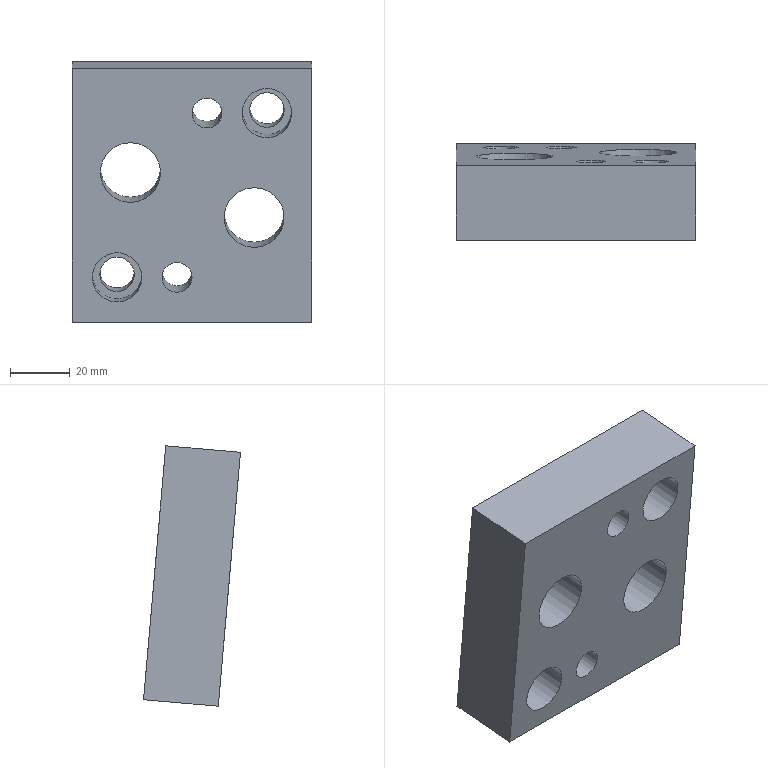Part | NX | features solid 2 | 1 solid | 20 faces | box 80 x 32.313 x 86.855 mm | volume 140365 mm3 | plane 10 | cylinder 10 | commonest cylinder face diameters 10 x2 11.5 x2 16.5 x2 20 x2 26 x2
STEP:
#1=CARTESIAN_POINT('',(208.,113.182,11.018));
#2=VERTEX_POINT('',#1);
#3=CARTESIAN_POINT('',(128.,113.182,11.018));
#4=VERTEX_POINT('',#3);
#5=CARTESIAN_POINT('',(208.,113.182,11.018));
#6=DIRECTION('',(-1.,0.,0.));
#7=VECTOR('',#6,1000.);
#8=LINE('',#5,#7);
#9=EDGE_CURVE('',#2,#4,#8,.T.);
#10=ORIENTED_EDGE('',*,*,#9,.F.);
#11=CARTESIAN_POINT('',(208.,138.087,13.197));
#12=VERTEX_POINT('',#11);
#13=CARTESIAN_POINT('',(208.,143.068,13.633));
#14=DIRECTION('',(0.,0.9962,0.08716));
#15=VECTOR('',#14,1000.);
#16=LINE('',#13,#15);
#17=EDGE_CURVE('',#12,#2,#16,.F.);
#18=ORIENTED_EDGE('',*,*,#17,.F.);
#19=CARTESIAN_POINT('',(128.,138.087,13.197));
#20=VERTEX_POINT('',#19);
#21=CARTESIAN_POINT('',(208.,138.087,13.197));
#22=DIRECTION('',(-1.,0.,0.));
#23=VECTOR('',#22,1000.);
#24=LINE('',#21,#23);
#25=EDGE_CURVE('',#12,#20,#24,.T.);
#26=ORIENTED_EDGE('',*,*,#25,.T.);
#27=CARTESIAN_POINT('',(128.,138.087,13.197));
#28=DIRECTION('',(0.,0.9962,0.08716));
#29=VECTOR('',#28,1000.);
#30=LINE('',#27,#29);
#31=EDGE_CURVE('',#20,#4,#30,.F.);
#32=ORIENTED_EDGE('',*,*,#31,.T.);
#33=EDGE_LOOP('',(#10,#18,#26,#32));
#34=FACE_BOUND('',#33,.T.);
#35=CARTESIAN_POINT('',(208.,143.068,13.633));
#36=DIRECTION('',(0.,0.08716,-0.9962));
#37=DIRECTION('',(0.,0.9962,0.08716));
#38=AXIS2_PLACEMENT_3D('',#35,#36,#37);
#39=PLANE('',#38);
#40=ADVANCED_FACE('',(#34),#39,.F.);
#41=CARTESIAN_POINT('',(128.,120.59,-73.658));
#42=VERTEX_POINT('',#41);
#43=CARTESIAN_POINT('',(128.,113.063,12.385));
#44=DIRECTION('',(0.,0.08716,-0.9962));
#45=VECTOR('',#44,1000.);
#46=LINE('',#43,#45);
#47=EDGE_CURVE('',#42,#4,#46,.F.);
#48=ORIENTED_EDGE('',*,*,#47,.T.);
#49=ORIENTED_EDGE('',*,*,#31,.F.);
#50=CARTESIAN_POINT('',(128.,145.495,-71.479));
#51=VERTEX_POINT('',#50);
#52=CARTESIAN_POINT('',(128.,137.967,14.563));
#53=DIRECTION('',(0.,0.08716,-0.9962));
#54=VECTOR('',#53,1000.);
#55=LINE('',#52,#54);
#56=EDGE_CURVE('',#51,#20,#55,.F.);
#57=ORIENTED_EDGE('',*,*,#56,.F.);
#58=CARTESIAN_POINT('',(128.,145.495,-71.479));
#59=DIRECTION('',(0.,0.9962,0.08716));
#60=VECTOR('',#59,1000.);
#61=LINE('',#58,#60);
#62=EDGE_CURVE('',#51,#42,#61,.F.);
#63=ORIENTED_EDGE('',*,*,#62,.T.);
#64=EDGE_LOOP('',(#48,#49,#57,#63));
#65=FACE_BOUND('',#64,.T.);
#66=CARTESIAN_POINT('',(128.,137.967,14.563));
#67=DIRECTION('',(1.,0.,0.));
#68=DIRECTION('',(0.,0.,-1.));
#69=AXIS2_PLACEMENT_3D('',#66,#67,#68);
#70=PLANE('',#69);
#71=ADVANCED_FACE('',(#65),#70,.F.);
#72=CARTESIAN_POINT('',(208.,120.59,-73.658));
#73=VERTEX_POINT('',#72);
#74=CARTESIAN_POINT('',(171.,120.59,-73.658));
#75=DIRECTION('',(1.,0.,0.));
#76=VECTOR('',#75,1000.);
#77=LINE('',#74,#76);
#78=EDGE_CURVE('',#42,#73,#77,.T.);
#79=ORIENTED_EDGE('',*,*,#78,.F.);
#80=ORIENTED_EDGE('',*,*,#62,.F.);
#81=CARTESIAN_POINT('',(208.,145.495,-71.479));
#82=VERTEX_POINT('',#81);
#83=CARTESIAN_POINT('',(171.,145.495,-71.479));
#84=DIRECTION('',(1.,0.,0.));
#85=VECTOR('',#84,1000.);
#86=LINE('',#83,#85);
#87=EDGE_CURVE('',#51,#82,#86,.T.);
#88=ORIENTED_EDGE('',*,*,#87,.T.);
#89=CARTESIAN_POINT('',(208.,279.982,-59.713));
#90=DIRECTION('',(0.,0.9962,0.08716));
#91=VECTOR('',#90,1000.);
#92=LINE('',#89,#91);
#93=EDGE_CURVE('',#82,#73,#92,.F.);
#94=ORIENTED_EDGE('',*,*,#93,.T.);
#95=EDGE_LOOP('',(#79,#80,#88,#94));
#96=FACE_BOUND('',#95,.T.);
#97=CARTESIAN_POINT('',(171.,279.982,-59.713));
#98=DIRECTION('',(0.,0.08716,-0.9962));
#99=DIRECTION('',(-1.,0.,0.));
#100=AXIS2_PLACEMENT_3D('',#97,#98,#99);
#101=PLANE('',#100);
#102=ADVANCED_FACE('',(#96),#101,.T.);
#103=CARTESIAN_POINT('',(208.,113.063,12.385));
#104=DIRECTION('',(0.,-0.08716,0.9962));
#105=VECTOR('',#104,1000.);
#106=LINE('',#103,#105);
#107=EDGE_CURVE('',#2,#73,#106,.F.);
#108=ORIENTED_EDGE('',*,*,#107,.T.);
#109=ORIENTED_EDGE('',*,*,#93,.F.);
#110=CARTESIAN_POINT('',(208.,142.543,-37.735));
#111=DIRECTION('',(0.,0.08716,-0.9962));
#112=VECTOR('',#111,1000.);
#113=LINE('',#110,#112);
#114=EDGE_CURVE('',#12,#82,#113,.T.);
#115=ORIENTED_EDGE('',*,*,#114,.F.);
#116=ORIENTED_EDGE('',*,*,#17,.T.);
#117=EDGE_LOOP('',(#108,#109,#115,#116));
#118=FACE_BOUND('',#117,.T.);
#119=CARTESIAN_POINT('',(208.,142.543,-37.735));
#120=DIRECTION('',(-1.,0.,0.));
#121=DIRECTION('',(0.,0.,1.));
#122=AXIS2_PLACEMENT_3D('',#119,#120,#121);
#123=PLANE('',#122);
#124=ADVANCED_FACE('',(#118),#123,.F.);
#125=CARTESIAN_POINT('',(193.,138.893,3.982));
#126=VERTEX_POINT('',#125);
#127=CARTESIAN_POINT('',(193.,139.394,-1.746));
#128=DIRECTION('',(0.,0.9962,0.08716));
#129=DIRECTION('',(0.,-0.08716,0.9962));
#130=AXIS2_PLACEMENT_3D('',#127,#128,#129);
#131=CIRCLE('',#130,5.75);
#132=EDGE_CURVE('',#126,#126,#131,.F.);
#133=ORIENTED_EDGE('',*,*,#132,.T.);
#134=EDGE_LOOP('',(#133));
#135=FACE_BOUND('',#134,.T.);
#136=CARTESIAN_POINT('',(173.,138.959,3.235));
#137=VERTEX_POINT('',#136);
#138=CARTESIAN_POINT('',(173.,139.394,-1.746));
#139=DIRECTION('',(0.,0.9962,0.08716));
#140=DIRECTION('',(0.,-0.08716,0.9962));
#141=AXIS2_PLACEMENT_3D('',#138,#139,#140);
#142=CIRCLE('',#141,5.);
#143=EDGE_CURVE('',#137,#137,#142,.F.);
#144=ORIENTED_EDGE('',*,*,#143,.T.);
#145=EDGE_LOOP('',(#144));
#146=FACE_BOUND('',#145,.T.);
#147=CARTESIAN_POINT('',(163.,143.752,-51.556));
#148=VERTEX_POINT('',#147);
#149=CARTESIAN_POINT('',(163.,144.188,-56.537));
#150=DIRECTION('',(0.,0.9962,0.08716));
#151=DIRECTION('',(0.,-0.08716,0.9962));
#152=AXIS2_PLACEMENT_3D('',#149,#150,#151);
#153=CIRCLE('',#152,5.);
#154=EDGE_CURVE('',#148,#148,#153,.F.);
#155=ORIENTED_EDGE('',*,*,#154,.T.);
#156=EDGE_LOOP('',(#155));
#157=FACE_BOUND('',#156,.T.);
#158=CARTESIAN_POINT('',(143.,143.687,-50.808));
#159=VERTEX_POINT('',#158);
#160=CARTESIAN_POINT('',(143.,144.188,-56.537));
#161=DIRECTION('',(0.,0.9962,0.08716));
#162=DIRECTION('',(0.,-0.08716,0.9962));
#163=AXIS2_PLACEMENT_3D('',#160,#161,#162);
#164=CIRCLE('',#163,5.75);
#165=EDGE_CURVE('',#159,#159,#164,.F.);
#166=ORIENTED_EDGE('',*,*,#165,.T.);
#167=EDGE_LOOP('',(#166));
#168=FACE_BOUND('',#167,.T.);
#169=CARTESIAN_POINT('',(147.466,139.995,-8.608));
#170=VERTEX_POINT('',#169);
#171=CARTESIAN_POINT('',(147.466,141.128,-21.558));
#172=DIRECTION('',(0.,0.9962,0.08716));
#173=DIRECTION('',(0.,-0.08716,0.9962));
#174=AXIS2_PLACEMENT_3D('',#171,#172,#173);
#175=CIRCLE('',#174,13.);
#176=EDGE_CURVE('',#170,#170,#175,.F.);
#177=ORIENTED_EDGE('',*,*,#176,.T.);
#178=EDGE_LOOP('',(#177));
#179=FACE_BOUND('',#178,.T.);
#180=CARTESIAN_POINT('',(188.737,141.307,-23.61));
#181=VERTEX_POINT('',#180);
#182=CARTESIAN_POINT('',(188.737,142.44,-36.56));
#183=DIRECTION('',(0.,0.9962,0.08716));
#184=DIRECTION('',(0.,-0.08716,0.9962));
#185=AXIS2_PLACEMENT_3D('',#182,#183,#184);
#186=CIRCLE('',#185,13.);
#187=EDGE_CURVE('',#181,#181,#186,.F.);
#188=ORIENTED_EDGE('',*,*,#187,.T.);
#189=EDGE_LOOP('',(#188));
#190=FACE_BOUND('',#189,.T.);
#191=ORIENTED_EDGE('',*,*,#25,.F.);
#192=ORIENTED_EDGE('',*,*,#114,.T.);
#193=ORIENTED_EDGE('',*,*,#87,.F.);
#194=ORIENTED_EDGE('',*,*,#56,.T.);
#195=EDGE_LOOP('',(#191,#192,#193,#194));
#196=FACE_BOUND('',#195,.T.);
#197=CARTESIAN_POINT('',(208.,137.967,14.563));
#198=DIRECTION('',(0.,0.9962,0.08716));
#199=DIRECTION('',(-1.,0.,0.));
#200=AXIS2_PLACEMENT_3D('',#197,#198,#199);
#201=PLANE('',#200);
#202=ADVANCED_FACE('',(#135,#146,#157,#168,#179,#190,#196),#201,.T.);
#203=CARTESIAN_POINT('',(178.,114.489,-3.925));
#204=VERTEX_POINT('',#203);
#205=CARTESIAN_POINT('',(173.,114.489,-3.925));
#206=DIRECTION('',(0.,0.9962,0.08716));
#207=DIRECTION('',(1.,0.,0.));
#208=AXIS2_PLACEMENT_3D('',#205,#206,#207);
#209=CIRCLE('',#208,5.);
#210=EDGE_CURVE('',#204,#204,#209,.T.);
#211=ORIENTED_EDGE('',*,*,#210,.T.);
#212=EDGE_LOOP('',(#211));
#213=FACE_BOUND('',#212,.T.);
#214=CARTESIAN_POINT('',(168.,119.283,-58.715));
#215=VERTEX_POINT('',#214);
#216=CARTESIAN_POINT('',(163.,119.283,-58.715));
#217=DIRECTION('',(0.,0.9962,0.08716));
#218=DIRECTION('',(1.,0.,0.));
#219=AXIS2_PLACEMENT_3D('',#216,#217,#218);
#220=CIRCLE('',#219,5.);
#221=EDGE_CURVE('',#215,#215,#220,.T.);
#222=ORIENTED_EDGE('',*,*,#221,.T.);
#223=EDGE_LOOP('',(#222));
#224=FACE_BOUND('',#223,.T.);
#225=CARTESIAN_POINT('',(151.25,119.283,-58.715));
#226=VERTEX_POINT('',#225);
#227=CARTESIAN_POINT('',(143.,119.283,-58.715));
#228=DIRECTION('',(0.,0.9962,0.08716));
#229=DIRECTION('',(1.,0.,0.));
#230=AXIS2_PLACEMENT_3D('',#227,#228,#229);
#231=CIRCLE('',#230,8.25);
#232=EDGE_CURVE('',#226,#226,#231,.T.);
#233=ORIENTED_EDGE('',*,*,#232,.T.);
#234=EDGE_LOOP('',(#233));
#235=FACE_BOUND('',#234,.T.);
#236=CARTESIAN_POINT('',(201.25,114.489,-3.925));
#237=VERTEX_POINT('',#236);
#238=CARTESIAN_POINT('',(193.,114.489,-3.925));
#239=DIRECTION('',(0.,0.9962,0.08716));
#240=DIRECTION('',(1.,0.,0.));
#241=AXIS2_PLACEMENT_3D('',#238,#239,#240);
#242=CIRCLE('',#241,8.25);
#243=EDGE_CURVE('',#237,#237,#242,.T.);
#244=ORIENTED_EDGE('',*,*,#243,.T.);
#245=EDGE_LOOP('',(#244));
#246=FACE_BOUND('',#245,.T.);
#247=CARTESIAN_POINT('',(147.466,115.351,-13.775));
#248=VERTEX_POINT('',#247);
#249=CARTESIAN_POINT('',(147.466,116.223,-23.737));
#250=DIRECTION('',(0.,0.9962,0.08716));
#251=DIRECTION('',(0.,-0.08716,0.9962));
#252=AXIS2_PLACEMENT_3D('',#249,#250,#251);
#253=CIRCLE('',#252,10.);
#254=EDGE_CURVE('',#248,#248,#253,.F.);
#255=ORIENTED_EDGE('',*,*,#254,.F.);
#256=EDGE_LOOP('',(#255));
#257=FACE_BOUND('',#256,.T.);
#258=CARTESIAN_POINT('',(188.737,116.664,-28.777));
#259=VERTEX_POINT('',#258);
#260=CARTESIAN_POINT('',(188.737,117.535,-38.739));
#261=DIRECTION('',(0.,0.9962,0.08716));
#262=DIRECTION('',(0.,-0.08716,0.9962));
#263=AXIS2_PLACEMENT_3D('',#260,#261,#262);
#264=CIRCLE('',#263,10.);
#265=EDGE_CURVE('',#259,#259,#264,.F.);
#266=ORIENTED_EDGE('',*,*,#265,.F.);
#267=EDGE_LOOP('',(#266));
#268=FACE_BOUND('',#267,.T.);
#269=ORIENTED_EDGE('',*,*,#9,.T.);
#270=ORIENTED_EDGE('',*,*,#47,.F.);
#271=ORIENTED_EDGE('',*,*,#78,.T.);
#272=ORIENTED_EDGE('',*,*,#107,.F.);
#273=EDGE_LOOP('',(#269,#270,#271,#272));
#274=FACE_BOUND('',#273,.T.);
#275=CARTESIAN_POINT('',(208.,113.063,12.385));
#276=DIRECTION('',(0.,0.9962,0.08716));
#277=DIRECTION('',(-1.,0.,0.));
#278=AXIS2_PLACEMENT_3D('',#275,#276,#277);
#279=PLANE('',#278);
#280=ADVANCED_FACE('',(#213,#224,#235,#246,#257,#268,#274),#279,.F.);
#281=ORIENTED_EDGE('',*,*,#265,.T.);
#282=EDGE_LOOP('',(#281));
#283=FACE_BOUND('',#282,.T.);
#284=CARTESIAN_POINT('',(188.737,138.331,-46.958));
#285=VERTEX_POINT('',#284);
#286=CARTESIAN_POINT('',(188.737,137.459,-36.996));
#287=DIRECTION('',(0.,-0.9962,-0.08716));
#288=DIRECTION('',(0.,0.08716,-0.9962));
#289=AXIS2_PLACEMENT_3D('',#286,#287,#288);
#290=CIRCLE('',#289,10.);
#291=EDGE_CURVE('',#285,#285,#290,.F.);
#292=ORIENTED_EDGE('',*,*,#291,.T.);
#293=EDGE_LOOP('',(#292));
#294=FACE_BOUND('',#293,.T.);
#295=CARTESIAN_POINT('',(188.737,75.948,-42.378));
#296=DIRECTION('',(0.,0.9962,0.08716));
#297=DIRECTION('',(0.,-0.08716,0.9962));
#298=AXIS2_PLACEMENT_3D('',#295,#296,#297);
#299=CYLINDRICAL_SURFACE('',#298,10.);
#300=ADVANCED_FACE('',(#283,#294),#299,.F.);
#301=ORIENTED_EDGE('',*,*,#291,.F.);
#302=EDGE_LOOP('',(#301));
#303=FACE_BOUND('',#302,.T.);
#304=CARTESIAN_POINT('',(175.737,137.459,-36.996));
#305=VERTEX_POINT('',#304);
#306=CARTESIAN_POINT('',(188.737,137.459,-36.996));
#307=DIRECTION('',(0.,-0.9962,-0.08716));
#308=DIRECTION('',(-1.,0.,0.));
#309=AXIS2_PLACEMENT_3D('',#306,#307,#308);
#310=CIRCLE('',#309,13.);
#311=EDGE_CURVE('',#305,#305,#310,.F.);
#312=ORIENTED_EDGE('',*,*,#311,.T.);
#313=EDGE_LOOP('',(#312));
#314=FACE_BOUND('',#313,.T.);
#315=CARTESIAN_POINT('',(188.737,137.459,-36.996));
#316=DIRECTION('',(0.,-0.9962,-0.08716));
#317=DIRECTION('',(0.,0.08716,-0.9962));
#318=AXIS2_PLACEMENT_3D('',#315,#316,#317);
#319=PLANE('',#318);
#320=ADVANCED_FACE('',(#303,#314),#319,.F.);
#321=ORIENTED_EDGE('',*,*,#187,.F.);
#322=EDGE_LOOP('',(#321));
#323=FACE_BOUND('',#322,.T.);
#324=ORIENTED_EDGE('',*,*,#311,.F.);
#325=EDGE_LOOP('',(#324));
#326=FACE_BOUND('',#325,.T.);
#327=CARTESIAN_POINT('',(188.737,127.497,-37.868));
#328=DIRECTION('',(0.,0.9962,0.08716));
#329=DIRECTION('',(0.,-0.08716,0.9962));
#330=AXIS2_PLACEMENT_3D('',#327,#328,#329);
#331=CYLINDRICAL_SURFACE('',#330,13.);
#332=ADVANCED_FACE('',(#323,#326),#331,.F.);
#333=ORIENTED_EDGE('',*,*,#254,.T.);
#334=EDGE_LOOP('',(#333));
#335=FACE_BOUND('',#334,.T.);
#336=CARTESIAN_POINT('',(147.466,137.018,-31.956));
#337=VERTEX_POINT('',#336);
#338=CARTESIAN_POINT('',(147.466,136.147,-21.994));
#339=DIRECTION('',(0.,-0.9962,-0.08716));
#340=DIRECTION('',(0.,0.08716,-0.9962));
#341=AXIS2_PLACEMENT_3D('',#338,#339,#340);
#342=CIRCLE('',#341,10.);
#343=EDGE_CURVE('',#337,#337,#342,.F.);
#344=ORIENTED_EDGE('',*,*,#343,.T.);
#345=EDGE_LOOP('',(#344));
#346=FACE_BOUND('',#345,.T.);
#347=CARTESIAN_POINT('',(147.466,74.636,-27.376));
#348=DIRECTION('',(0.,0.9962,0.08716));
#349=DIRECTION('',(0.,-0.08716,0.9962));
#350=AXIS2_PLACEMENT_3D('',#347,#348,#349);
#351=CYLINDRICAL_SURFACE('',#350,10.);
#352=ADVANCED_FACE('',(#335,#346),#351,.F.);
#353=ORIENTED_EDGE('',*,*,#343,.F.);
#354=EDGE_LOOP('',(#353));
#355=FACE_BOUND('',#354,.T.);
#356=CARTESIAN_POINT('',(134.466,136.147,-21.994));
#357=VERTEX_POINT('',#356);
#358=CARTESIAN_POINT('',(147.466,136.147,-21.994));
#359=DIRECTION('',(0.,-0.9962,-0.08716));
#360=DIRECTION('',(-1.,0.,0.));
#361=AXIS2_PLACEMENT_3D('',#358,#359,#360);
#362=CIRCLE('',#361,13.);
#363=EDGE_CURVE('',#357,#357,#362,.F.);
#364=ORIENTED_EDGE('',*,*,#363,.T.);
#365=EDGE_LOOP('',(#364));
#366=FACE_BOUND('',#365,.T.);
#367=CARTESIAN_POINT('',(147.466,136.147,-21.994));
#368=DIRECTION('',(0.,-0.9962,-0.08716));
#369=DIRECTION('',(0.,0.08716,-0.9962));
#370=AXIS2_PLACEMENT_3D('',#367,#368,#369);
#371=PLANE('',#370);
#372=ADVANCED_FACE('',(#355,#366),#371,.F.);
#373=ORIENTED_EDGE('',*,*,#176,.F.);
#374=EDGE_LOOP('',(#373));
#375=FACE_BOUND('',#374,.T.);
#376=ORIENTED_EDGE('',*,*,#363,.F.);
#377=EDGE_LOOP('',(#376));
#378=FACE_BOUND('',#377,.T.);
#379=CARTESIAN_POINT('',(147.466,126.185,-22.866));
#380=DIRECTION('',(0.,0.9962,0.08716));
#381=DIRECTION('',(0.,-0.08716,0.9962));
#382=AXIS2_PLACEMENT_3D('',#379,#380,#381);
#383=CYLINDRICAL_SURFACE('',#382,13.);
#384=ADVANCED_FACE('',(#375,#378),#383,.F.);
#385=ORIENTED_EDGE('',*,*,#243,.F.);
#386=EDGE_LOOP('',(#385));
#387=FACE_BOUND('',#386,.T.);
#388=CARTESIAN_POINT('',(201.25,126.444,-2.879));
#389=VERTEX_POINT('',#388);
#390=CARTESIAN_POINT('',(193.,126.444,-2.879));
#391=DIRECTION('',(0.,0.9962,0.08716));
#392=DIRECTION('',(1.,0.,0.));
#393=AXIS2_PLACEMENT_3D('',#390,#391,#392);
#394=CIRCLE('',#393,8.25);
#395=EDGE_CURVE('',#389,#389,#394,.T.);
#396=ORIENTED_EDGE('',*,*,#395,.T.);
#397=EDGE_LOOP('',(#396));
#398=FACE_BOUND('',#397,.T.);
#399=CARTESIAN_POINT('',(193.,114.489,-3.925));
#400=DIRECTION('',(0.,0.9962,0.08716));
#401=DIRECTION('',(1.,0.,0.));
#402=AXIS2_PLACEMENT_3D('',#399,#400,#401);
#403=CYLINDRICAL_SURFACE('',#402,8.25);
#404=ADVANCED_FACE('',(#387,#398),#403,.F.);
#405=CARTESIAN_POINT('',(198.75,126.444,-2.879));
#406=VERTEX_POINT('',#405);
#407=CARTESIAN_POINT('',(193.,126.444,-2.879));
#408=DIRECTION('',(0.,0.9962,0.08716));
#409=DIRECTION('',(1.,0.,0.));
#410=AXIS2_PLACEMENT_3D('',#407,#408,#409);
#411=CIRCLE('',#410,5.75);
#412=EDGE_CURVE('',#406,#406,#411,.T.);
#413=ORIENTED_EDGE('',*,*,#412,.T.);
#414=EDGE_LOOP('',(#413));
#415=FACE_BOUND('',#414,.T.);
#416=ORIENTED_EDGE('',*,*,#395,.F.);
#417=EDGE_LOOP('',(#416));
#418=FACE_BOUND('',#417,.T.);
#419=CARTESIAN_POINT('',(193.,126.444,-2.879));
#420=DIRECTION('',(0.,0.9962,0.08716));
#421=DIRECTION('',(1.,0.,0.));
#422=AXIS2_PLACEMENT_3D('',#419,#420,#421);
#423=PLANE('',#422);
#424=ADVANCED_FACE('',(#415,#418),#423,.F.);
#425=ORIENTED_EDGE('',*,*,#232,.F.);
#426=EDGE_LOOP('',(#425));
#427=FACE_BOUND('',#426,.T.);
#428=CARTESIAN_POINT('',(151.25,131.237,-57.67));
#429=VERTEX_POINT('',#428);
#430=CARTESIAN_POINT('',(143.,131.237,-57.67));
#431=DIRECTION('',(0.,0.9962,0.08716));
#432=DIRECTION('',(1.,0.,0.));
#433=AXIS2_PLACEMENT_3D('',#430,#431,#432);
#434=CIRCLE('',#433,8.25);
#435=EDGE_CURVE('',#429,#429,#434,.T.);
#436=ORIENTED_EDGE('',*,*,#435,.T.);
#437=EDGE_LOOP('',(#436));
#438=FACE_BOUND('',#437,.T.);
#439=CARTESIAN_POINT('',(143.,119.283,-58.715));
#440=DIRECTION('',(0.,0.9962,0.08716));
#441=DIRECTION('',(1.,0.,0.));
#442=AXIS2_PLACEMENT_3D('',#439,#440,#441);
#443=CYLINDRICAL_SURFACE('',#442,8.25);
#444=ADVANCED_FACE('',(#427,#438),#443,.F.);
#445=CARTESIAN_POINT('',(148.75,131.237,-57.67));
#446=VERTEX_POINT('',#445);
#447=CARTESIAN_POINT('',(143.,131.237,-57.67));
#448=DIRECTION('',(0.,0.9962,0.08716));
#449=DIRECTION('',(1.,0.,0.));
#450=AXIS2_PLACEMENT_3D('',#447,#448,#449);
#451=CIRCLE('',#450,5.75);
#452=EDGE_CURVE('',#446,#446,#451,.T.);
#453=ORIENTED_EDGE('',*,*,#452,.T.);
#454=EDGE_LOOP('',(#453));
#455=FACE_BOUND('',#454,.T.);
#456=ORIENTED_EDGE('',*,*,#435,.F.);
#457=EDGE_LOOP('',(#456));
#458=FACE_BOUND('',#457,.T.);
#459=CARTESIAN_POINT('',(143.,131.237,-57.67));
#460=DIRECTION('',(0.,0.9962,0.08716));
#461=DIRECTION('',(1.,0.,0.));
#462=AXIS2_PLACEMENT_3D('',#459,#460,#461);
#463=PLANE('',#462);
#464=ADVANCED_FACE('',(#455,#458),#463,.F.);
#465=ORIENTED_EDGE('',*,*,#452,.F.);
#466=EDGE_LOOP('',(#465));
#467=FACE_BOUND('',#466,.T.);
#468=ORIENTED_EDGE('',*,*,#165,.F.);
#469=EDGE_LOOP('',(#468));
#470=FACE_BOUND('',#469,.T.);
#471=CARTESIAN_POINT('',(143.,119.283,-58.715));
#472=DIRECTION('',(0.,0.9962,0.08716));
#473=DIRECTION('',(1.,0.,0.));
#474=AXIS2_PLACEMENT_3D('',#471,#472,#473);
#475=CYLINDRICAL_SURFACE('',#474,5.75);
#476=ADVANCED_FACE('',(#467,#470),#475,.F.);
#477=ORIENTED_EDGE('',*,*,#221,.F.);
#478=EDGE_LOOP('',(#477));
#479=FACE_BOUND('',#478,.T.);
#480=ORIENTED_EDGE('',*,*,#154,.F.);
#481=EDGE_LOOP('',(#480));
#482=FACE_BOUND('',#481,.T.);
#483=CARTESIAN_POINT('',(163.,119.283,-58.715));
#484=DIRECTION('',(0.,0.9962,0.08716));
#485=DIRECTION('',(1.,0.,0.));
#486=AXIS2_PLACEMENT_3D('',#483,#484,#485);
#487=CYLINDRICAL_SURFACE('',#486,5.);
#488=ADVANCED_FACE('',(#479,#482),#487,.F.);
#489=ORIENTED_EDGE('',*,*,#210,.F.);
#490=EDGE_LOOP('',(#489));
#491=FACE_BOUND('',#490,.T.);
#492=ORIENTED_EDGE('',*,*,#143,.F.);
#493=EDGE_LOOP('',(#492));
#494=FACE_BOUND('',#493,.T.);
#495=CARTESIAN_POINT('',(173.,114.489,-3.925));
#496=DIRECTION('',(0.,0.9962,0.08716));
#497=DIRECTION('',(1.,0.,0.));
#498=AXIS2_PLACEMENT_3D('',#495,#496,#497);
#499=CYLINDRICAL_SURFACE('',#498,5.);
#500=ADVANCED_FACE('',(#491,#494),#499,.F.);
#501=ORIENTED_EDGE('',*,*,#412,.F.);
#502=EDGE_LOOP('',(#501));
#503=FACE_BOUND('',#502,.T.);
#504=ORIENTED_EDGE('',*,*,#132,.F.);
#505=EDGE_LOOP('',(#504));
#506=FACE_BOUND('',#505,.T.);
#507=CARTESIAN_POINT('',(193.,114.489,-3.925));
#508=DIRECTION('',(0.,0.9962,0.08716));
#509=DIRECTION('',(1.,0.,0.));
#510=AXIS2_PLACEMENT_3D('',#507,#508,#509);
#511=CYLINDRICAL_SURFACE('',#510,5.75);
#512=ADVANCED_FACE('',(#503,#506),#511,.F.);
#513=CLOSED_SHELL('',(#40,#71,#102,#124,#202,#280,#300,#320,#332,#352,#372,#384,#404,#424,#444,#464,#476,#488,#500,#512));
#514=MANIFOLD_SOLID_BREP('',#513);
#515=(LENGTH_UNIT()NAMED_UNIT(*)SI_UNIT(.MILLI.,.METRE.));
#516=UNCERTAINTY_MEASURE_WITH_UNIT(LENGTH_MEASURE(0.00001),#515,'','');
#517=(NAMED_UNIT(*)PLANE_ANGLE_UNIT()SI_UNIT($,.RADIAN.));
#518=(NAMED_UNIT(*)SI_UNIT($,.STERADIAN.)SOLID_ANGLE_UNIT());
#519=(GEOMETRIC_REPRESENTATION_CONTEXT(3)GLOBAL_UNCERTAINTY_ASSIGNED_CONTEXT((#516))GLOBAL_UNIT_ASSIGNED_CONTEXT((#515,#517,#518))REPRESENTATION_CONTEXT('',''));
#520=ADVANCED_BREP_SHAPE_REPRESENTATION('',(#514),#519);